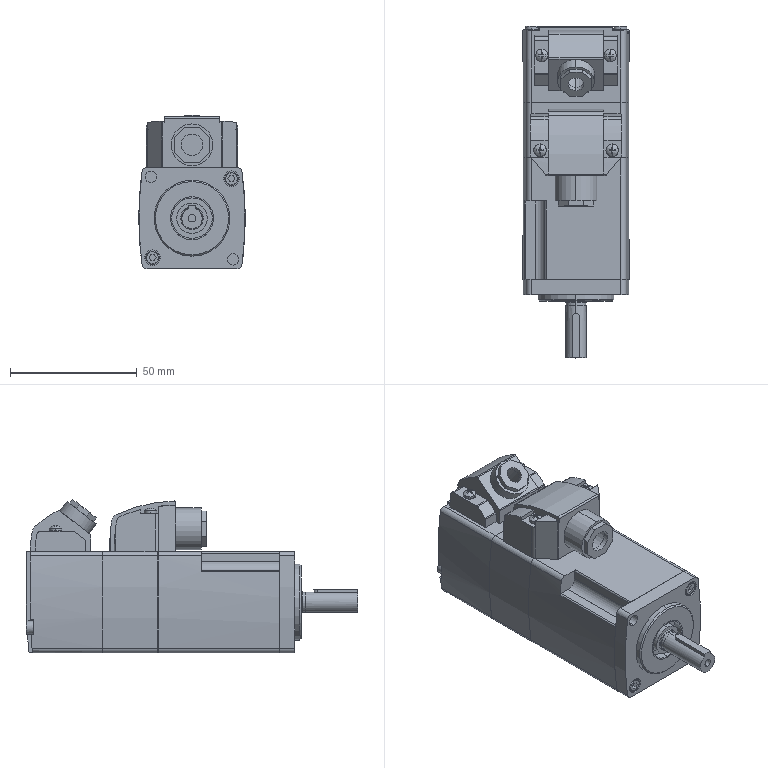Part | SolidWorks | 10 solids | 536 faces | box 42.009 x 131.188 x 60.7 mm | volume 192000 mm3 | plane 298 | cylinder 204 | spline 32 | cone 2 | commonest cylinder face diameters 1.2 x26 4 x26 2.8 x8 5 x8 5.232 x8 268.2 x8